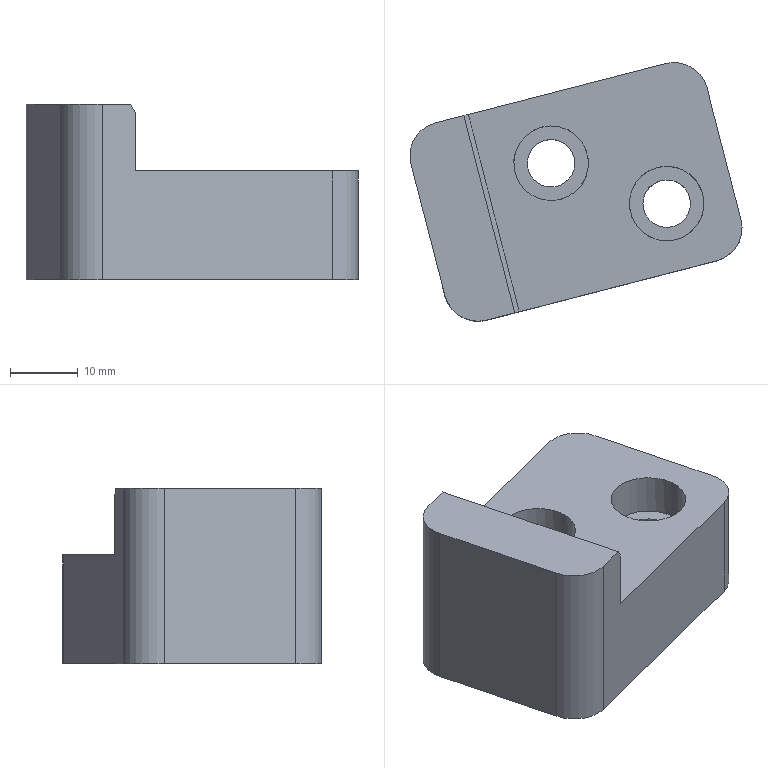Part | STEP file | 车灯-后视镜_id182_x_t | 1 solid | 19 faces | box 48.889 x 38.111 x 25.8 mm | volume 22170 mm3 | plane 11 | cylinder 8 | commonest cylinder face diameters 10 x4 7 x2 11 x2
STEP:
#1=CARTESIAN_POINT('',(-62.077,58.719,-41.286));
#2=VERTEX_POINT('',#1);
#3=CARTESIAN_POINT('',(-57.08,39.353,-41.286));
#4=VERTEX_POINT('',#3);
#5=CARTESIAN_POINT('',(-68.422,83.311,-41.286));
#6=DIRECTION('',(0.2498,-0.9683,0.));
#7=VECTOR('',#6,1.);
#8=LINE('',#5,#7);
#9=EDGE_CURVE('',#2,#4,#8,.T.);
#10=ORIENTED_EDGE('',*,*,#9,.F.);
#11=CARTESIAN_POINT('',(-62.077,58.719,-25.286));
#12=VERTEX_POINT('',#11);
#13=CARTESIAN_POINT('',(-62.077,58.719,35.852));
#14=DIRECTION('',(0.,0.,1.));
#15=VECTOR('',#14,1.);
#16=LINE('',#13,#15);
#17=EDGE_CURVE('',#2,#12,#16,.T.);
#18=ORIENTED_EDGE('',*,*,#17,.T.);
#19=CARTESIAN_POINT('',(-57.08,39.353,-25.286));
#20=VERTEX_POINT('',#19);
#21=CARTESIAN_POINT('',(-68.422,83.311,-25.286));
#22=DIRECTION('',(0.2498,-0.9683,0.));
#23=VECTOR('',#22,1.);
#24=LINE('',#21,#23);
#25=EDGE_CURVE('',#12,#20,#24,.T.);
#26=ORIENTED_EDGE('',*,*,#25,.T.);
#27=CARTESIAN_POINT('',(-57.08,39.353,35.852));
#28=DIRECTION('',(0.,0.,-1.));
#29=VECTOR('',#28,1.);
#30=LINE('',#27,#29);
#31=EDGE_CURVE('',#20,#4,#30,.T.);
#32=ORIENTED_EDGE('',*,*,#31,.T.);
#33=EDGE_LOOP('',(#10,#18,#26,#32));
#34=FACE_OUTER_BOUND('',#33,.T.);
#35=CARTESIAN_POINT('',(-61.294,55.685,35.852));
#36=DIRECTION('',(-0.9683,-0.2498,0.));
#37=DIRECTION('',(-0.2498,0.9683,0.));
#38=AXIS2_PLACEMENT_3D('',#35,#36,#37);
#39=PLANE('',#38);
#40=ADVANCED_FACE('',(#34),#39,.F.);
#41=CARTESIAN_POINT('',(-60.673,33.262,-41.286));
#42=VERTEX_POINT('',#41);
#43=CARTESIAN_POINT('',(-94.566,24.517,-41.286));
#44=VERTEX_POINT('',#43);
#45=CARTESIAN_POINT('',(-70.356,30.764,-41.286));
#46=DIRECTION('',(-0.9683,-0.2498,0.));
#47=VECTOR('',#46,1.);
#48=LINE('',#45,#47);
#49=EDGE_CURVE('',#42,#44,#48,.T.);
#50=ORIENTED_EDGE('',*,*,#49,.F.);
#51=CARTESIAN_POINT('',(-60.673,33.262,-25.286));
#52=VERTEX_POINT('',#51);
#53=CARTESIAN_POINT('',(-60.673,33.262,-25.286));
#54=DIRECTION('',(0.,0.,1.));
#55=VECTOR('',#54,1.);
#56=LINE('',#53,#55);
#57=EDGE_CURVE('',#42,#52,#56,.T.);
#58=ORIENTED_EDGE('',*,*,#57,.T.);
#59=CARTESIAN_POINT('',(-89.725,25.766,-25.286));
#60=VERTEX_POINT('',#59);
#61=CARTESIAN_POINT('',(-70.36,30.763,-25.286));
#62=DIRECTION('',(0.9683,0.2498,0.));
#63=VECTOR('',#62,1.);
#64=LINE('',#61,#63);
#65=EDGE_CURVE('',#60,#52,#64,.T.);
#66=ORIENTED_EDGE('',*,*,#65,.F.);
#67=CARTESIAN_POINT('',(-89.725,25.766,-16.686));
#68=VERTEX_POINT('',#67);
#69=CARTESIAN_POINT('',(-89.725,25.766,-25.286));
#70=DIRECTION('',(0.,0.,-1.));
#71=VECTOR('',#70,1.);
#72=LINE('',#69,#71);
#73=EDGE_CURVE('',#68,#60,#72,.T.);
#74=ORIENTED_EDGE('',*,*,#73,.F.);
#75=CARTESIAN_POINT('',(-90.396,25.593,-15.486));
#76=VERTEX_POINT('',#75);
#77=CARTESIAN_POINT('',(-90.395,25.594,-15.487));
#78=DIRECTION('',(-0.4841,-0.1249,0.866));
#79=VECTOR('',#78,1.);
#80=LINE('',#77,#79);
#81=EDGE_CURVE('',#68,#76,#80,.T.);
#82=ORIENTED_EDGE('',*,*,#81,.T.);
#83=CARTESIAN_POINT('',(-94.566,24.517,-15.486));
#84=VERTEX_POINT('',#83);
#85=CARTESIAN_POINT('',(-70.356,30.764,-15.486));
#86=DIRECTION('',(-0.9683,-0.2498,0.));
#87=VECTOR('',#86,1.);
#88=LINE('',#85,#87);
#89=EDGE_CURVE('',#76,#84,#88,.T.);
#90=ORIENTED_EDGE('',*,*,#89,.T.);
#91=CARTESIAN_POINT('',(-94.566,24.517,-25.286));
#92=DIRECTION('',(0.,0.,-1.));
#93=VECTOR('',#92,1.);
#94=LINE('',#91,#93);
#95=EDGE_CURVE('',#84,#44,#94,.T.);
#96=ORIENTED_EDGE('',*,*,#95,.T.);
#97=EDGE_LOOP('',(#50,#58,#66,#74,#82,#90,#96));
#98=FACE_OUTER_BOUND('',#97,.T.);
#99=CARTESIAN_POINT('',(-70.36,30.763,-25.286));
#100=DIRECTION('',(0.2498,-0.9683,0.));
#101=DIRECTION('',(-0.9683,-0.2498,0.));
#102=AXIS2_PLACEMENT_3D('',#99,#100,#101);
#103=PLANE('',#102);
#104=ADVANCED_FACE('',(#98),#103,.T.);
#105=CARTESIAN_POINT('',(-105.652,47.476,-15.486));
#106=VERTEX_POINT('',#105);
#107=CARTESIAN_POINT('',(-100.657,28.11,-15.486));
#108=VERTEX_POINT('',#107);
#109=CARTESIAN_POINT('',(-111.995,72.069,-15.486));
#110=DIRECTION('',(0.2498,-0.9683,0.));
#111=VECTOR('',#110,1.);
#112=LINE('',#109,#111);
#113=EDGE_CURVE('',#106,#108,#112,.T.);
#114=ORIENTED_EDGE('',*,*,#113,.F.);
#115=CARTESIAN_POINT('',(-105.652,47.476,-41.286));
#116=VERTEX_POINT('',#115);
#117=CARTESIAN_POINT('',(-105.652,47.476,-25.286));
#118=DIRECTION('',(0.,0.,-1.));
#119=VECTOR('',#118,1.);
#120=LINE('',#117,#119);
#121=EDGE_CURVE('',#106,#116,#120,.T.);
#122=ORIENTED_EDGE('',*,*,#121,.T.);
#123=CARTESIAN_POINT('',(-100.657,28.11,-41.286));
#124=VERTEX_POINT('',#123);
#125=CARTESIAN_POINT('',(-111.995,72.069,-41.286));
#126=DIRECTION('',(0.2498,-0.9683,0.));
#127=VECTOR('',#126,1.);
#128=LINE('',#125,#127);
#129=EDGE_CURVE('',#116,#124,#128,.T.);
#130=ORIENTED_EDGE('',*,*,#129,.T.);
#131=CARTESIAN_POINT('',(-100.657,28.11,-25.286));
#132=DIRECTION('',(0.,0.,1.));
#133=VECTOR('',#132,1.);
#134=LINE('',#131,#133);
#135=EDGE_CURVE('',#124,#108,#134,.T.);
#136=ORIENTED_EDGE('',*,*,#135,.T.);
#137=EDGE_LOOP('',(#114,#122,#130,#136));
#138=FACE_OUTER_BOUND('',#137,.T.);
#139=CARTESIAN_POINT('',(-111.995,72.069,-25.286));
#140=DIRECTION('',(0.9683,0.2498,0.));
#141=DIRECTION('',(0.2498,-0.9683,0.));
#142=AXIS2_PLACEMENT_3D('',#139,#140,#141);
#143=PLANE('',#142);
#144=ADVANCED_FACE('',(#138),#143,.F.);
#145=CARTESIAN_POINT('',(-68.168,62.311,-41.286));
#146=VERTEX_POINT('',#145);
#147=CARTESIAN_POINT('',(-102.06,53.566,-41.286));
#148=VERTEX_POINT('',#147);
#149=CARTESIAN_POINT('',(-77.851,59.813,-41.286));
#150=DIRECTION('',(-0.9683,-0.2498,0.));
#151=VECTOR('',#150,1.);
#152=LINE('',#149,#151);
#153=EDGE_CURVE('',#146,#148,#152,.T.);
#154=ORIENTED_EDGE('',*,*,#153,.T.);
#155=CARTESIAN_POINT('',(-102.06,53.566,-15.486));
#156=VERTEX_POINT('',#155);
#157=CARTESIAN_POINT('',(-102.06,53.566,-25.286));
#158=DIRECTION('',(0.,0.,1.));
#159=VECTOR('',#158,1.);
#160=LINE('',#157,#159);
#161=EDGE_CURVE('',#148,#156,#160,.T.);
#162=ORIENTED_EDGE('',*,*,#161,.T.);
#163=CARTESIAN_POINT('',(-97.889,54.642,-15.486));
#164=VERTEX_POINT('',#163);
#165=CARTESIAN_POINT('',(-77.851,59.813,-15.486));
#166=DIRECTION('',(-0.9683,-0.2498,0.));
#167=VECTOR('',#166,1.);
#168=LINE('',#165,#167);
#169=EDGE_CURVE('',#164,#156,#168,.T.);
#170=ORIENTED_EDGE('',*,*,#169,.F.);
#171=CARTESIAN_POINT('',(-97.218,54.816,-16.686));
#172=VERTEX_POINT('',#171);
#173=CARTESIAN_POINT('',(-97.888,54.643,-15.486));
#174=DIRECTION('',(0.4841,0.1249,-0.866));
#175=VECTOR('',#174,1.);
#176=LINE('',#173,#175);
#177=EDGE_CURVE('',#164,#172,#176,.T.);
#178=ORIENTED_EDGE('',*,*,#177,.T.);
#179=CARTESIAN_POINT('',(-97.218,54.816,-25.286));
#180=VERTEX_POINT('',#179);
#181=CARTESIAN_POINT('',(-97.218,54.816,-25.286));
#182=DIRECTION('',(0.,0.,1.));
#183=VECTOR('',#182,1.);
#184=LINE('',#181,#183);
#185=EDGE_CURVE('',#180,#172,#184,.T.);
#186=ORIENTED_EDGE('',*,*,#185,.F.);
#187=CARTESIAN_POINT('',(-68.168,62.311,-25.286));
#188=VERTEX_POINT('',#187);
#189=CARTESIAN_POINT('',(-77.851,59.813,-25.286));
#190=DIRECTION('',(-0.9683,-0.2498,0.));
#191=VECTOR('',#190,1.);
#192=LINE('',#189,#191);
#193=EDGE_CURVE('',#188,#180,#192,.T.);
#194=ORIENTED_EDGE('',*,*,#193,.F.);
#195=CARTESIAN_POINT('',(-68.168,62.311,-25.286));
#196=DIRECTION('',(0.,0.,-1.));
#197=VECTOR('',#196,1.);
#198=LINE('',#195,#197);
#199=EDGE_CURVE('',#188,#146,#198,.T.);
#200=ORIENTED_EDGE('',*,*,#199,.T.);
#201=EDGE_LOOP('',(#154,#162,#170,#178,#186,#194,#200));
#202=FACE_OUTER_BOUND('',#201,.T.);
#203=CARTESIAN_POINT('',(-77.851,59.813,-25.286));
#204=DIRECTION('',(0.2498,-0.9683,0.));
#205=DIRECTION('',(-0.9683,-0.2498,0.));
#206=AXIS2_PLACEMENT_3D('',#203,#204,#205);
#207=PLANE('',#206);
#208=ADVANCED_FACE('',(#202),#207,.F.);
#209=CARTESIAN_POINT('',(-71.512,41.697,-41.286));
#210=VERTEX_POINT('',#209);
#211=CARTESIAN_POINT('',(-68.012,41.697,-41.286));
#212=DIRECTION('',(0.,0.,1.));
#213=DIRECTION('',(-1.,0.,0.));
#214=AXIS2_PLACEMENT_3D('',#211,#212,#213);
#215=CIRCLE('',#214,3.5);
#216=EDGE_CURVE('',#210,#210,#215,.T.);
#217=ORIENTED_EDGE('',*,*,#216,.T.);
#218=EDGE_LOOP('',(#217));
#219=FACE_BOUND('',#218,.T.);
#220=CARTESIAN_POINT('',(-88.534,47.635,-41.286));
#221=VERTEX_POINT('',#220);
#222=CARTESIAN_POINT('',(-85.034,47.635,-41.286));
#223=DIRECTION('',(0.,0.,1.));
#224=DIRECTION('',(-1.,0.,0.));
#225=AXIS2_PLACEMENT_3D('',#222,#223,#224);
#226=CIRCLE('',#225,3.5);
#227=EDGE_CURVE('',#221,#221,#226,.T.);
#228=ORIENTED_EDGE('',*,*,#227,.T.);
#229=EDGE_LOOP('',(#228));
#230=FACE_BOUND('',#229,.T.);
#231=ORIENTED_EDGE('',*,*,#129,.F.);
#232=CARTESIAN_POINT('',(-100.81,48.725,-41.286));
#233=DIRECTION('',(0.,0.,-1.));
#234=DIRECTION('',(1.,0.,0.));
#235=AXIS2_PLACEMENT_3D('',#232,#233,#234);
#236=CIRCLE('',#235,5.);
#237=EDGE_CURVE('',#116,#148,#236,.T.);
#238=ORIENTED_EDGE('',*,*,#237,.T.);
#239=ORIENTED_EDGE('',*,*,#153,.F.);
#240=CARTESIAN_POINT('',(-66.919,57.47,-41.286));
#241=DIRECTION('',(0.,0.,-1.));
#242=DIRECTION('',(1.,0.,0.));
#243=AXIS2_PLACEMENT_3D('',#240,#241,#242);
#244=CIRCLE('',#243,5.);
#245=EDGE_CURVE('',#146,#2,#244,.T.);
#246=ORIENTED_EDGE('',*,*,#245,.T.);
#247=ORIENTED_EDGE('',*,*,#9,.T.);
#248=CARTESIAN_POINT('',(-61.922,38.104,-41.286));
#249=DIRECTION('',(0.,0.,-1.));
#250=DIRECTION('',(1.,0.,0.));
#251=AXIS2_PLACEMENT_3D('',#248,#249,#250);
#252=CIRCLE('',#251,5.);
#253=EDGE_CURVE('',#4,#42,#252,.T.);
#254=ORIENTED_EDGE('',*,*,#253,.T.);
#255=ORIENTED_EDGE('',*,*,#49,.T.);
#256=CARTESIAN_POINT('',(-95.815,29.359,-41.286));
#257=DIRECTION('',(0.,0.,-1.));
#258=DIRECTION('',(1.,0.,0.));
#259=AXIS2_PLACEMENT_3D('',#256,#257,#258);
#260=CIRCLE('',#259,5.);
#261=EDGE_CURVE('',#44,#124,#260,.T.);
#262=ORIENTED_EDGE('',*,*,#261,.T.);
#263=EDGE_LOOP('',(#231,#238,#239,#246,#247,#254,#255,#262));
#264=FACE_BOUND('',#263,.T.);
#265=CARTESIAN_POINT('',(-82.947,79.564,-41.286));
#266=DIRECTION('',(0.,0.,1.));
#267=DIRECTION('',(-0.8752,-0.4837,0.));
#268=AXIS2_PLACEMENT_3D('',#265,#266,#267);
#269=PLANE('',#268);
#270=ADVANCED_FACE('',(#219,#230,#264),#269,.F.);
#271=ORIENTED_EDGE('',*,*,#169,.T.);
#272=CARTESIAN_POINT('',(-100.81,48.725,-15.486));
#273=DIRECTION('',(0.,0.,1.));
#274=DIRECTION('',(1.,0.,0.));
#275=AXIS2_PLACEMENT_3D('',#272,#273,#274);
#276=CIRCLE('',#275,5.);
#277=EDGE_CURVE('',#156,#106,#276,.T.);
#278=ORIENTED_EDGE('',*,*,#277,.T.);
#279=ORIENTED_EDGE('',*,*,#113,.T.);
#280=CARTESIAN_POINT('',(-95.815,29.359,-15.486));
#281=DIRECTION('',(0.,0.,1.));
#282=DIRECTION('',(1.,0.,0.));
#283=AXIS2_PLACEMENT_3D('',#280,#281,#282);
#284=CIRCLE('',#283,5.);
#285=EDGE_CURVE('',#108,#84,#284,.T.);
#286=ORIENTED_EDGE('',*,*,#285,.T.);
#287=ORIENTED_EDGE('',*,*,#89,.F.);
#288=CARTESIAN_POINT('',(-97.889,54.643,-15.486));
#289=DIRECTION('',(-0.2498,0.9683,0.));
#290=VECTOR('',#289,1.);
#291=LINE('',#288,#290);
#292=EDGE_CURVE('',#76,#164,#291,.T.);
#293=ORIENTED_EDGE('',*,*,#292,.T.);
#294=EDGE_LOOP('',(#271,#278,#279,#286,#287,#293));
#295=FACE_OUTER_BOUND('',#294,.T.);
#296=CARTESIAN_POINT('',(-82.947,79.564,-15.486));
#297=DIRECTION('',(0.,0.,1.));
#298=DIRECTION('',(-0.8752,-0.4837,0.));
#299=AXIS2_PLACEMENT_3D('',#296,#297,#298);
#300=PLANE('',#299);
#301=ADVANCED_FACE('',(#295),#300,.T.);
#302=CARTESIAN_POINT('',(-69.385,47.023,-25.286));
#303=VERTEX_POINT('',#302);
#304=CARTESIAN_POINT('',(-68.012,41.697,-25.286));
#305=DIRECTION('',(0.,0.,-1.));
#306=DIRECTION('',(-0.2497,0.9683,0.));
#307=AXIS2_PLACEMENT_3D('',#304,#305,#306);
#308=CIRCLE('',#307,5.5);
#309=EDGE_CURVE('',#303,#303,#308,.T.);
#310=ORIENTED_EDGE('',*,*,#309,.T.);
#311=EDGE_LOOP('',(#310));
#312=FACE_BOUND('',#311,.T.);
#313=CARTESIAN_POINT('',(-86.407,52.96,-25.286));
#314=VERTEX_POINT('',#313);
#315=CARTESIAN_POINT('',(-85.034,47.635,-25.286));
#316=DIRECTION('',(0.,0.,-1.));
#317=DIRECTION('',(-0.2497,0.9683,0.));
#318=AXIS2_PLACEMENT_3D('',#315,#316,#317);
#319=CIRCLE('',#318,5.5);
#320=EDGE_CURVE('',#314,#314,#319,.T.);
#321=ORIENTED_EDGE('',*,*,#320,.T.);
#322=EDGE_LOOP('',(#321));
#323=FACE_BOUND('',#322,.T.);
#324=ORIENTED_EDGE('',*,*,#25,.F.);
#325=CARTESIAN_POINT('',(-66.919,57.47,-25.286));
#326=DIRECTION('',(0.,0.,1.));
#327=DIRECTION('',(1.,0.,0.));
#328=AXIS2_PLACEMENT_3D('',#325,#326,#327);
#329=CIRCLE('',#328,5.);
#330=EDGE_CURVE('',#12,#188,#329,.T.);
#331=ORIENTED_EDGE('',*,*,#330,.T.);
#332=ORIENTED_EDGE('',*,*,#193,.T.);
#333=CARTESIAN_POINT('',(-102.312,74.567,-25.286));
#334=DIRECTION('',(0.2498,-0.9683,0.));
#335=VECTOR('',#334,1.);
#336=LINE('',#333,#335);
#337=EDGE_CURVE('',#180,#60,#336,.T.);
#338=ORIENTED_EDGE('',*,*,#337,.T.);
#339=ORIENTED_EDGE('',*,*,#65,.T.);
#340=CARTESIAN_POINT('',(-61.922,38.104,-25.286));
#341=DIRECTION('',(0.,0.,1.));
#342=DIRECTION('',(1.,0.,0.));
#343=AXIS2_PLACEMENT_3D('',#340,#341,#342);
#344=CIRCLE('',#343,5.);
#345=EDGE_CURVE('',#52,#20,#344,.T.);
#346=ORIENTED_EDGE('',*,*,#345,.T.);
#347=EDGE_LOOP('',(#324,#331,#332,#338,#339,#346));
#348=FACE_BOUND('',#347,.T.);
#349=CARTESIAN_POINT('',(-102.671,74.475,-25.286));
#350=DIRECTION('',(0.,0.,1.));
#351=DIRECTION('',(-0.8752,-0.4837,0.));
#352=AXIS2_PLACEMENT_3D('',#349,#350,#351);
#353=PLANE('',#352);
#354=ADVANCED_FACE('',(#312,#323,#348),#353,.T.);
#355=ORIENTED_EDGE('',*,*,#185,.T.);
#356=CARTESIAN_POINT('',(-89.725,25.766,-16.686));
#357=DIRECTION('',(0.2498,-0.9683,0.));
#358=VECTOR('',#357,1.);
#359=LINE('',#356,#358);
#360=EDGE_CURVE('',#172,#68,#359,.T.);
#361=ORIENTED_EDGE('',*,*,#360,.T.);
#362=ORIENTED_EDGE('',*,*,#73,.T.);
#363=ORIENTED_EDGE('',*,*,#337,.F.);
#364=EDGE_LOOP('',(#355,#361,#362,#363));
#365=FACE_OUTER_BOUND('',#364,.T.);
#366=CARTESIAN_POINT('',(-102.312,74.567,-25.286));
#367=DIRECTION('',(0.9683,0.2498,0.));
#368=DIRECTION('',(0.2498,-0.9683,0.));
#369=AXIS2_PLACEMENT_3D('',#366,#367,#368);
#370=PLANE('',#369);
#371=ADVANCED_FACE('',(#365),#370,.T.);
#372=ORIENTED_EDGE('',*,*,#81,.F.);
#373=ORIENTED_EDGE('',*,*,#360,.F.);
#374=ORIENTED_EDGE('',*,*,#177,.F.);
#375=ORIENTED_EDGE('',*,*,#292,.F.);
#376=EDGE_LOOP('',(#372,#373,#374,#375));
#377=FACE_OUTER_BOUND('',#376,.T.);
#378=CARTESIAN_POINT('',(-102.984,74.395,-15.486));
#379=DIRECTION('',(-0.8386,-0.2163,-0.5));
#380=DIRECTION('',(-0.5121,0.,0.8589));
#381=AXIS2_PLACEMENT_3D('',#378,#379,#380);
#382=PLANE('',#381);
#383=ADVANCED_FACE('',(#377),#382,.F.);
#384=ORIENTED_EDGE('',*,*,#277,.F.);
#385=ORIENTED_EDGE('',*,*,#161,.F.);
#386=ORIENTED_EDGE('',*,*,#237,.F.);
#387=ORIENTED_EDGE('',*,*,#121,.F.);
#388=EDGE_LOOP('',(#384,#385,#386,#387));
#389=FACE_OUTER_BOUND('',#388,.T.);
#390=CARTESIAN_POINT('',(-100.81,48.725,-25.286));
#391=DIRECTION('',(0.,0.,-1.));
#392=DIRECTION('',(-1.,0.,0.));
#393=AXIS2_PLACEMENT_3D('',#390,#391,#392);
#394=CYLINDRICAL_SURFACE('',#393,5.);
#395=ADVANCED_FACE('',(#389),#394,.T.);
#396=ORIENTED_EDGE('',*,*,#330,.F.);
#397=ORIENTED_EDGE('',*,*,#17,.F.);
#398=ORIENTED_EDGE('',*,*,#245,.F.);
#399=ORIENTED_EDGE('',*,*,#199,.F.);
#400=EDGE_LOOP('',(#396,#397,#398,#399));
#401=FACE_OUTER_BOUND('',#400,.T.);
#402=CARTESIAN_POINT('',(-66.919,57.47,-25.286));
#403=DIRECTION('',(0.,0.,-1.));
#404=DIRECTION('',(-1.,0.,0.));
#405=AXIS2_PLACEMENT_3D('',#402,#403,#404);
#406=CYLINDRICAL_SURFACE('',#405,5.);
#407=ADVANCED_FACE('',(#401),#406,.T.);
#408=ORIENTED_EDGE('',*,*,#345,.F.);
#409=ORIENTED_EDGE('',*,*,#57,.F.);
#410=ORIENTED_EDGE('',*,*,#253,.F.);
#411=ORIENTED_EDGE('',*,*,#31,.F.);
#412=EDGE_LOOP('',(#408,#409,#410,#411));
#413=FACE_OUTER_BOUND('',#412,.T.);
#414=CARTESIAN_POINT('',(-61.922,38.104,35.852));
#415=DIRECTION('',(0.,0.,1.));
#416=DIRECTION('',(1.,0.,0.));
#417=AXIS2_PLACEMENT_3D('',#414,#415,#416);
#418=CYLINDRICAL_SURFACE('',#417,5.);
#419=ADVANCED_FACE('',(#413),#418,.T.);
#420=ORIENTED_EDGE('',*,*,#285,.F.);
#421=ORIENTED_EDGE('',*,*,#135,.F.);
#422=ORIENTED_EDGE('',*,*,#261,.F.);
#423=ORIENTED_EDGE('',*,*,#95,.F.);
#424=EDGE_LOOP('',(#420,#421,#422,#423));
#425=FACE_OUTER_BOUND('',#424,.T.);
#426=CARTESIAN_POINT('',(-95.815,29.359,-25.286));
#427=DIRECTION('',(0.,0.,1.));
#428=DIRECTION('',(1.,0.,0.));
#429=AXIS2_PLACEMENT_3D('',#426,#427,#428);
#430=CYLINDRICAL_SURFACE('',#429,5.);
#431=ADVANCED_FACE('',(#425),#430,.T.);
#432=CARTESIAN_POINT('',(-88.534,47.635,-31.286));
#433=VERTEX_POINT('',#432);
#434=CARTESIAN_POINT('',(-85.034,47.635,-31.286));
#435=DIRECTION('',(0.,0.,1.));
#436=DIRECTION('',(-1.,0.,0.));
#437=AXIS2_PLACEMENT_3D('',#434,#435,#436);
#438=CIRCLE('',#437,3.5);
#439=EDGE_CURVE('',#433,#433,#438,.T.);
#440=ORIENTED_EDGE('',*,*,#439,.T.);
#441=EDGE_LOOP('',(#440));
#442=FACE_BOUND('',#441,.T.);
#443=ORIENTED_EDGE('',*,*,#227,.F.);
#444=EDGE_LOOP('',(#443));
#445=FACE_BOUND('',#444,.T.);
#446=CARTESIAN_POINT('',(-85.034,47.635,-35.286));
#447=DIRECTION('',(0.,0.,1.));
#448=DIRECTION('',(0.2497,-0.9683,0.));
#449=AXIS2_PLACEMENT_3D('',#446,#447,#448);
#450=CYLINDRICAL_SURFACE('',#449,3.5);
#451=ADVANCED_FACE('',(#442,#445),#450,.F.);
#452=ORIENTED_EDGE('',*,*,#439,.F.);
#453=EDGE_LOOP('',(#452));
#454=FACE_BOUND('',#453,.T.);
#455=CARTESIAN_POINT('',(-90.534,47.635,-31.286));
#456=VERTEX_POINT('',#455);
#457=CARTESIAN_POINT('',(-85.034,47.635,-31.286));
#458=DIRECTION('',(0.,0.,1.));
#459=DIRECTION('',(-1.,0.,0.));
#460=AXIS2_PLACEMENT_3D('',#457,#458,#459);
#461=CIRCLE('',#460,5.5);
#462=EDGE_CURVE('',#456,#456,#461,.T.);
#463=ORIENTED_EDGE('',*,*,#462,.T.);
#464=EDGE_LOOP('',(#463));
#465=FACE_BOUND('',#464,.T.);
#466=CARTESIAN_POINT('',(-85.034,47.635,-31.286));
#467=DIRECTION('',(0.,0.,-1.));
#468=DIRECTION('',(-0.2497,0.9683,0.));
#469=AXIS2_PLACEMENT_3D('',#466,#467,#468);
#470=PLANE('',#469);
#471=ADVANCED_FACE('',(#454,#465),#470,.F.);
#472=ORIENTED_EDGE('',*,*,#462,.F.);
#473=EDGE_LOOP('',(#472));
#474=FACE_BOUND('',#473,.T.);
#475=ORIENTED_EDGE('',*,*,#320,.F.);
#476=EDGE_LOOP('',(#475));
#477=FACE_BOUND('',#476,.T.);
#478=CARTESIAN_POINT('',(-85.034,47.635,-25.286));
#479=DIRECTION('',(0.,0.,-1.));
#480=DIRECTION('',(-0.2497,0.9683,0.));
#481=AXIS2_PLACEMENT_3D('',#478,#479,#480);
#482=CYLINDRICAL_SURFACE('',#481,5.5);
#483=ADVANCED_FACE('',(#474,#477),#482,.F.);
#484=CARTESIAN_POINT('',(-71.512,41.697,-31.286));
#485=VERTEX_POINT('',#484);
#486=CARTESIAN_POINT('',(-68.012,41.697,-31.286));
#487=DIRECTION('',(0.,0.,1.));
#488=DIRECTION('',(-1.,0.,0.));
#489=AXIS2_PLACEMENT_3D('',#486,#487,#488);
#490=CIRCLE('',#489,3.5);
#491=EDGE_CURVE('',#485,#485,#490,.T.);
#492=ORIENTED_EDGE('',*,*,#491,.T.);
#493=EDGE_LOOP('',(#492));
#494=FACE_BOUND('',#493,.T.);
#495=ORIENTED_EDGE('',*,*,#216,.F.);
#496=EDGE_LOOP('',(#495));
#497=FACE_BOUND('',#496,.T.);
#498=CARTESIAN_POINT('',(-68.012,41.697,-35.286));
#499=DIRECTION('',(0.,0.,1.));
#500=DIRECTION('',(0.2497,-0.9683,0.));
#501=AXIS2_PLACEMENT_3D('',#498,#499,#500);
#502=CYLINDRICAL_SURFACE('',#501,3.5);
#503=ADVANCED_FACE('',(#494,#497),#502,.F.);
#504=ORIENTED_EDGE('',*,*,#491,.F.);
#505=EDGE_LOOP('',(#504));
#506=FACE_BOUND('',#505,.T.);
#507=CARTESIAN_POINT('',(-73.512,41.697,-31.286));
#508=VERTEX_POINT('',#507);
#509=CARTESIAN_POINT('',(-68.012,41.697,-31.286));
#510=DIRECTION('',(0.,0.,1.));
#511=DIRECTION('',(-1.,0.,0.));
#512=AXIS2_PLACEMENT_3D('',#509,#510,#511);
#513=CIRCLE('',#512,5.5);
#514=EDGE_CURVE('',#508,#508,#513,.T.);
#515=ORIENTED_EDGE('',*,*,#514,.T.);
#516=EDGE_LOOP('',(#515));
#517=FACE_BOUND('',#516,.T.);
#518=CARTESIAN_POINT('',(-68.012,41.697,-31.286));
#519=DIRECTION('',(0.,0.,-1.));
#520=DIRECTION('',(-0.2497,0.9683,0.));
#521=AXIS2_PLACEMENT_3D('',#518,#519,#520);
#522=PLANE('',#521);
#523=ADVANCED_FACE('',(#506,#517),#522,.F.);
#524=ORIENTED_EDGE('',*,*,#514,.F.);
#525=EDGE_LOOP('',(#524));
#526=FACE_BOUND('',#525,.T.);
#527=ORIENTED_EDGE('',*,*,#309,.F.);
#528=EDGE_LOOP('',(#527));
#529=FACE_BOUND('',#528,.T.);
#530=CARTESIAN_POINT('',(-68.012,41.697,-25.286));
#531=DIRECTION('',(0.,0.,-1.));
#532=DIRECTION('',(-0.2497,0.9683,0.));
#533=AXIS2_PLACEMENT_3D('',#530,#531,#532);
#534=CYLINDRICAL_SURFACE('',#533,5.5);
#535=ADVANCED_FACE('',(#526,#529),#534,.F.);
#536=CLOSED_SHELL('',(#40,#104,#144,#208,#270,#301,#354,#371,#383,#395,#407,#419,#431,#451,#471,#483,#503,#523,#535));
#537=MANIFOLD_SOLID_BREP('',#536);
#538=(LENGTH_UNIT()NAMED_UNIT(*)SI_UNIT(.MILLI.,.METRE.));
#539=UNCERTAINTY_MEASURE_WITH_UNIT(LENGTH_MEASURE(0.00002),#538,'','');
#540=(NAMED_UNIT(*)PLANE_ANGLE_UNIT()SI_UNIT($,.RADIAN.));
#541=PLANE_ANGLE_MEASURE_WITH_UNIT(PLANE_ANGLE_MEASURE(0.01745),#540);
#542=DIMENSIONAL_EXPONENTS(0.,0.,0.,0.,0.,0.,0.);
#543=(CONVERSION_BASED_UNIT('DEGREE',#541)NAMED_UNIT(#542)PLANE_ANGLE_UNIT());
#544=(NAMED_UNIT(*)SI_UNIT($,.STERADIAN.)SOLID_ANGLE_UNIT());
#545=(GEOMETRIC_REPRESENTATION_CONTEXT(3)GLOBAL_UNCERTAINTY_ASSIGNED_CONTEXT((#539))GLOBAL_UNIT_ASSIGNED_CONTEXT((#538,#543,#544))REPRESENTATION_CONTEXT('',''));
#546=ADVANCED_BREP_SHAPE_REPRESENTATION('',(#537),#545);